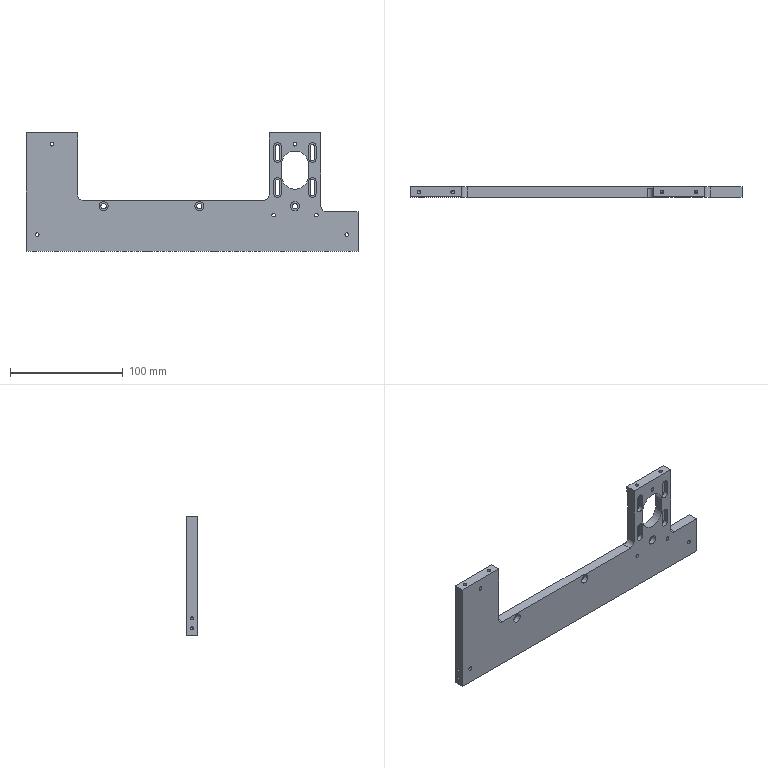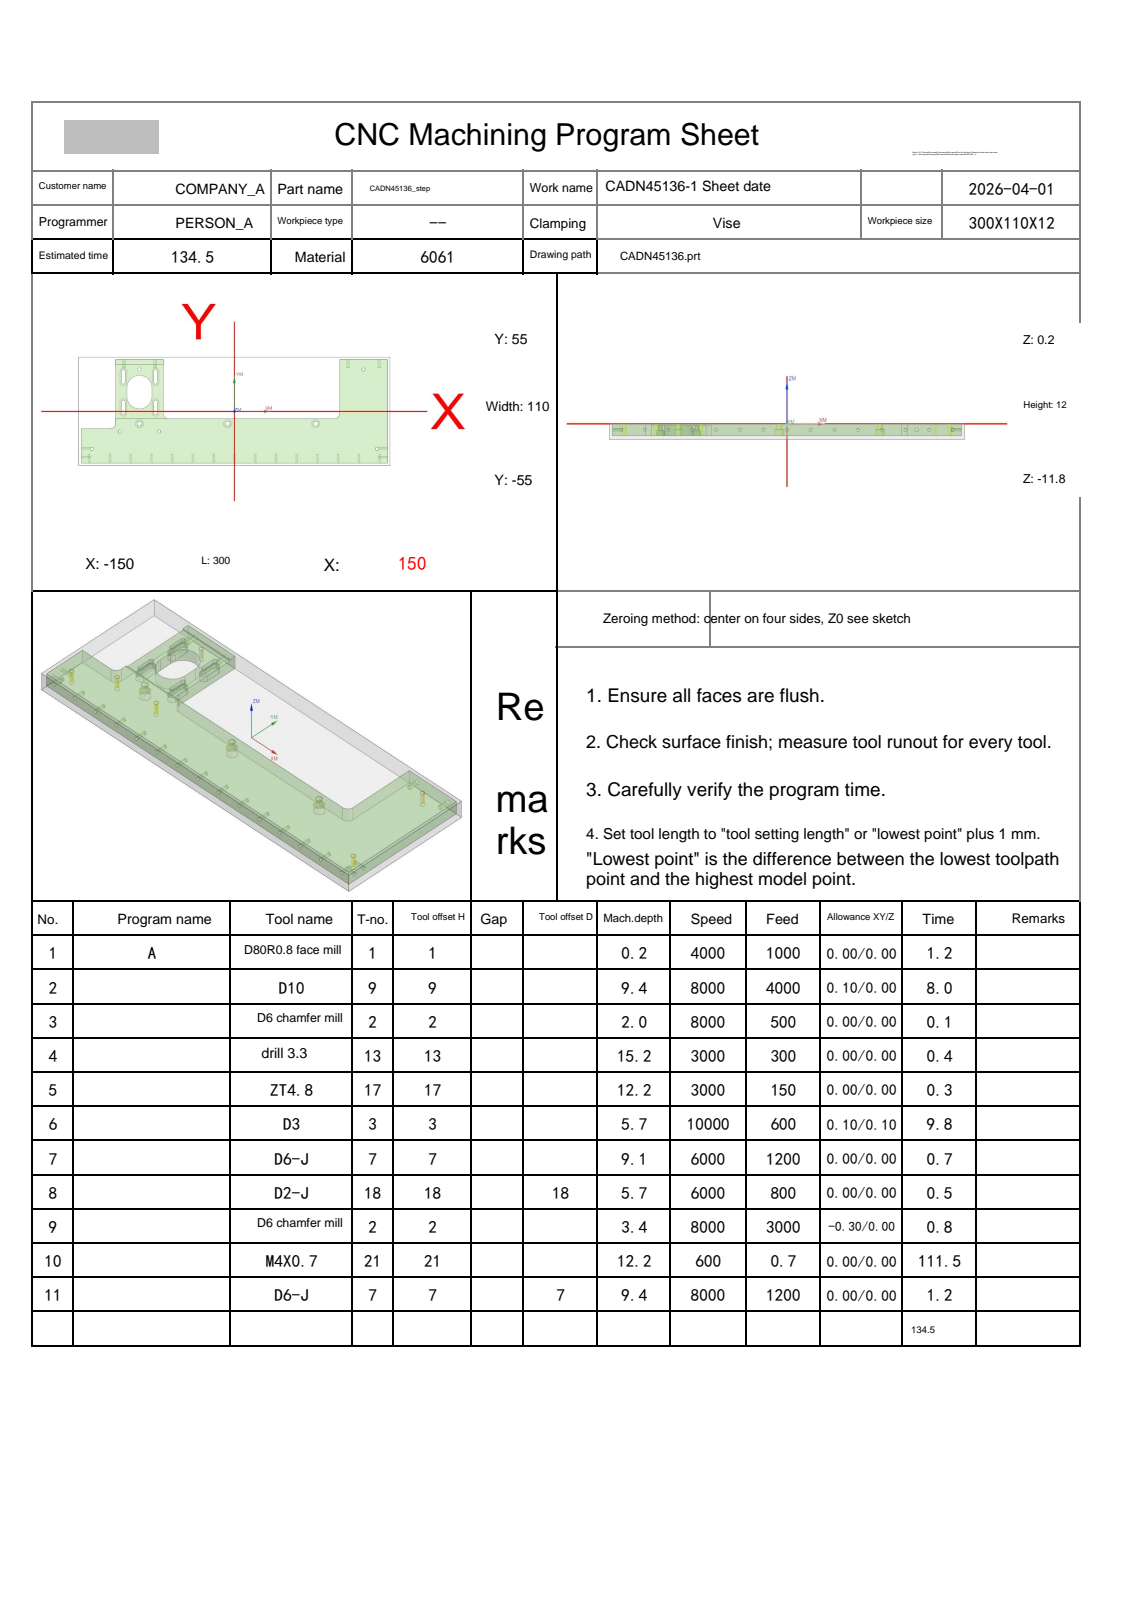NC program | NX | posted by the shop | part box 295 x 9 x 105 mm
Lines 3256 to 4696 of 7463:
N6 T03 M06
(D3  D=3. R=0. H=03 ce=0.10 di=0.10)
G00 G90 G54 X-76.1 Y4. M03 S10000
G43 H03 Z20.
M08
Z-.5
G01 Y-1.55 Z-.519 F600.
X-76.095 Y-1.605
X-76.055 Y-1.645 Z-.52
X-76. Y-1.65
X-75.945 Y-1.645
X-75.905 Y-1.605
X-75.9 Y-1.55
Y9.55 Z-.559
X-75.905 Y9.605
X-75.945 Y9.645
X-76. Y9.65 Z-.56
X-76.055 Y9.645
X-76.095 Y9.605
X-76.1 Y9.55
Y-1.55 Z-.599
X-76.095 Y-1.605
X-76.055 Y-1.645
X-76. Y-1.65
X-75.945 Y-1.645
X-75.905 Y-1.605 Z-.6
X-75.9 Y-1.55
Y9.55 Z-.638
X-75.905 Y9.605 Z-.639
X-75.945 Y9.645
X-76. Y9.65
X-76.055 Y9.645
X-76.095 Y9.605
X-76.1 Y9.55
Y-1.55 Z-.678
X-76.095 Y-1.605
X-76.055 Y-1.645
X-76. Y-1.65 Z-.679
X-75.945 Y-1.645
X-75.905 Y-1.605
X-75.9 Y-1.55
Y9.55 Z-.718
X-75.905 Y9.605
X-75.945 Y9.645
X-76. Y9.65
X-76.055 Y9.645
X-76.095 Y9.605 Z-.719
X-76.1 Y9.55
Y-1.55 Z-.757
X-76.095 Y-1.605 Z-.758
X-76.055 Y-1.645
X-76. Y-1.65
X-75.945 Y-1.645
X-75.905 Y-1.605
X-75.9 Y-1.55
Y9.55 Z-.797
X-75.905 Y9.605
X-75.945 Y9.645
X-76. Y9.65 Z-.798
X-76.055 Y9.645
X-76.095 Y9.605
X-76.1 Y9.55
Y-1.55 Z-.837
X-76.095 Y-1.605
X-76.055 Y-1.645
X-76. Y-1.65
X-75.945 Y-1.645
X-75.905 Y-1.605 Z-.838
X-75.9 Y-1.55
Y9.55 Z-.876
X-75.905 Y9.605 Z-.877
X-75.945 Y9.645
X-76. Y9.65
X-76.055 Y9.645
X-76.095 Y9.605
X-76.1 Y9.55 Z-.878
Y-1.55 Z-.916
X-76.095 Y-1.605
X-76.055 Y-1.645
X-76. Y-1.65 Z-.917
X-75.945 Y-1.645
X-75.905 Y-1.605
X-75.9 Y-1.55
Y9.55 Z-.956
X-75.905 Y9.605
X-75.945 Y9.645
X-76. Y9.65
X-76.055 Y9.645 Z-.957
X-76.095 Y9.605
X-76.1 Y9.55
Y-1.55 Z-.995
X-76.095 Y-1.605 Z-.996
X-76.055 Y-1.645
X-76. Y-1.65
X-75.945 Y-1.645
X-75.905 Y-1.605
X-75.9 Y-1.55 Z-.997
Y9.55 Z-1.035
X-75.905 Y9.605
X-75.945 Y9.645 Z-1.036
X-76. Y9.65
X-76.055 Y9.645
X-76.095 Y9.605
X-76.1 Y9.55
Y-1.55 Z-1.075
X-76.095 Y-1.605
X-76.055 Y-1.645
X-76. Y-1.65
X-75.945 Y-1.645 Z-1.076
X-75.905 Y-1.605
X-75.9 Y-1.55
Y9.55 Z-1.115
X-75.905 Y9.605
X-75.945 Y9.645
X-76. Y9.65
X-76.055 Y9.645
X-76.095 Y9.605
X-76.1 Y9.55 Z-1.116
Y-1.55 Z-1.154
X-76.095 Y-1.605
X-76.055 Y-1.645 Z-1.155
X-76. Y-1.65
X-75.945 Y-1.645
X-75.905 Y-1.605
X-75.9 Y-1.55
Y9.55 Z-1.194
X-75.905 Y9.605
X-75.945 Y9.645
X-76. Y9.65
X-76.055 Y9.645 Z-1.195
X-76.095 Y9.605
X-76.1 Y9.55
Y-1.55 Z-1.234
X-76.095 Y-1.605
X-76.055 Y-1.645
X-76. Y-1.65
X-75.945 Y-1.645
X-75.905 Y-1.605
X-75.9 Y-1.55 Z-1.235
Y9.55 Z-1.273
X-75.905 Y9.605
X-75.945 Y9.645 Z-1.274
X-76. Y9.65
X-76.055 Y9.645
X-76.095 Y9.605
X-76.1 Y9.55
Y-1.55 Z-1.313
X-76.095 Y-1.605
X-76.055 Y-1.645
X-76. Y-1.65
X-75.945 Y-1.645 Z-1.314
X-75.905 Y-1.605
X-75.9 Y-1.55
Y9.55 Z-1.353
X-75.905 Y9.605
X-75.945 Y9.645
X-76. Y9.65
X-76.055 Y9.645
X-76.095 Y9.605 Z-1.354
X-76.1 Y9.55
Y-1.55 Z-1.392
X-76.095 Y-1.605
X-76.055 Y-1.645 Z-1.393
X-76. Y-1.65
X-75.945 Y-1.645
X-75.905 Y-1.605
X-75.9 Y-1.55
Y9.55 Z-1.432
X-75.905 Y9.605
X-75.945 Y9.645
X-76. Y9.65 Z-1.433
X-76.055 Y9.645
X-76.095 Y9.605
X-76.1 Y9.55
Y-1.55 Z-1.472
X-76.095 Y-1.605
X-76.055 Y-1.645
X-76. Y-1.65
X-75.945 Y-1.645
X-75.905 Y-1.605 Z-1.473
X-75.9 Y-1.55
Y9.55 Z-1.511
X-75.905 Y9.605 Z-1.512
X-75.945 Y9.645
X-76. Y9.65
X-76.055 Y9.645
X-76.095 Y9.605
X-76.1 Y9.55
Y-1.55 Z-1.551
X-76.095 Y-1.605
X-76.055 Y-1.645
X-76. Y-1.65 Z-1.552
X-75.945 Y-1.645
X-75.905 Y-1.605
X-75.9 Y-1.55
Y9.55 Z-1.591
X-75.905 Y9.605
X-75.945 Y9.645
X-76. Y9.65
X-76.055 Y9.645
X-76.095 Y9.605 Z-1.592
X-76.1 Y9.55
Y-1.55 Z-1.63
X-76.095 Y-1.605 Z-1.631
X-76.055 Y-1.645
X-76. Y-1.65
X-75.945 Y-1.645
X-75.905 Y-1.605
X-75.9 Y-1.55
Y9.55 Z-1.67
X-75.905 Y9.605
X-75.945 Y9.645
X-76. Y9.65 Z-1.671
X-76.055 Y9.645
X-76.095 Y9.605
X-76.1 Y9.55
Y-1.55 Z-1.71
X-76.095 Y-1.605
X-76.055 Y-1.645
X-76. Y-1.65
X-75.945 Y-1.645 Z-1.711
X-75.905 Y-1.605
X-75.9 Y-1.55
Y9.55 Z-1.749
X-75.905 Y9.605 Z-1.75
X-75.945 Y9.645
X-76. Y9.65
X-76.055 Y9.645
X-76.095 Y9.605
X-76.1 Y9.55 Z-1.751
Y-1.55 Z-1.789
X-76.095 Y-1.605
X-76.055 Y-1.645 Z-1.79
X-76. Y-1.65
X-75.945 Y-1.645
X-75.905 Y-1.605
X-75.9 Y-1.55
Y9.55 Z-1.829
X-75.905 Y9.605
X-75.945 Y9.645
X-76. Y9.65
X-76.055 Y9.645 Z-1.83
X-76.095 Y9.605
X-76.1 Y9.55
Y-1.55 Z-1.869
X-76.095 Y-1.605
X-76.055 Y-1.645
X-76. Y-1.65
X-75.945 Y-1.645
X-75.905 Y-1.605
X-75.9 Y-1.55 Z-1.87
Y9.55 Z-1.908
X-75.905 Y9.605
X-75.945 Y9.645 Z-1.909
X-76. Y9.65
X-76.055 Y9.645
X-76.095 Y9.605
X-76.1 Y9.55
Y-1.55 Z-1.948
X-76.095 Y-1.605
X-76.055 Y-1.645
X-76. Y-1.65
X-75.945 Y-1.645 Z-1.949
X-75.905 Y-1.605
X-75.9 Y-1.55
Y9.55 Z-1.988
X-75.905 Y9.605
X-75.945 Y9.645
X-76. Y9.65
X-76.055 Y9.645
X-76.095 Y9.605
X-76.1 Y9.55 Z-1.989
Y-1.55 Z-2.027
X-76.095 Y-1.605
X-76.055 Y-1.645 Z-2.028
X-76. Y-1.65
X-75.945 Y-1.645
X-75.905 Y-1.605
X-75.9 Y-1.55
Y9.55 Z-2.067
X-75.905 Y9.605
X-75.945 Y9.645
X-76. Y9.65
X-76.055 Y9.645 Z-2.068
X-76.095 Y9.605
X-76.1 Y9.55
Y-1.55 Z-2.107
X-76.095 Y-1.605
X-76.055 Y-1.645
X-76. Y-1.65
X-75.945 Y-1.645
X-75.905 Y-1.605 Z-2.108
X-75.9 Y-1.55
Y9.55 Z-2.146
X-75.905 Y9.605
X-75.945 Y9.645 Z-2.147
X-76. Y9.65
X-76.055 Y9.645
X-76.095 Y9.605
X-76.1 Y9.55
Y-1.55 Z-2.186
X-76.095 Y-1.605
X-76.055 Y-1.645
X-76. Y-1.65 Z-2.187
X-75.945 Y-1.645
X-75.905 Y-1.605
X-75.9 Y-1.55
Y9.55 Z-2.226
X-75.905 Y9.605
X-75.945 Y9.645
X-76. Y9.65
X-76.055 Y9.645
X-76.095 Y9.605 Z-2.227
X-76.1 Y9.55
Y-1.55 Z-2.265
X-76.095 Y-1.605 Z-2.266
X-76.055 Y-1.645
X-76. Y-1.65
X-75.945 Y-1.645
X-75.905 Y-1.605
X-75.9 Y-1.55
Y9.55 Z-2.305
X-75.905 Y9.605
X-75.945 Y9.645
X-76. Y9.65 Z-2.306
X-76.055 Y9.645
X-76.095 Y9.605
X-76.1 Y9.55
Y-1.55 Z-2.345
X-76.095 Y-1.605
X-76.055 Y-1.645
X-76. Y-1.65
X-75.945 Y-1.645
X-75.905 Y-1.605 Z-2.346
X-75.9 Y-1.55
Y9.55 Z-2.384
X-75.905 Y9.605 Z-2.385
X-75.945 Y9.645
X-76. Y9.65
X-76.055 Y9.645
X-76.095 Y9.605
X-76.1 Y9.55
Y-1.55 Z-2.424
X-76.095 Y-1.605
X-76.055 Y-1.645
X-76. Y-1.65 Z-2.425
X-75.945 Y-1.645
X-75.905 Y-1.605
X-75.9 Y-1.55
Y9.55 Z-2.464
X-75.905 Y9.605
X-75.945 Y9.645
X-76. Y9.65
X-76.055 Y9.645
X-76.095 Y9.605 Z-2.465
X-76.1 Y9.55
Y-1.55 Z-2.503
X-76.095 Y-1.605 Z-2.504
X-76.055 Y-1.645
X-76. Y-1.65
X-75.945 Y-1.645
X-75.905 Y-1.605
X-75.9 Y-1.55 Z-2.505
Y9.55 Z-2.543
X-75.905 Y9.605
X-75.945 Y9.645
X-76. Y9.65 Z-2.544
X-76.055 Y9.645
X-76.095 Y9.605
X-76.1 Y9.55
Y-1.55 Z-2.583
X-76.095 Y-1.605
X-76.055 Y-1.645
X-76. Y-1.65
X-75.945 Y-1.645 Z-2.584
X-75.905 Y-1.605
X-75.9 Y-1.55
Y9.55 Z-2.622
X-75.905 Y9.605 Z-2.623
X-75.945 Y9.645
X-76. Y9.65
X-76.055 Y9.645
X-76.095 Y9.605
X-76.1 Y9.55 Z-2.624
Y-1.55 Z-2.662
X-76.095 Y-1.605
X-76.055 Y-1.645 Z-2.663
X-76. Y-1.65
X-75.945 Y-1.645
X-75.905 Y-1.605
X-75.9 Y-1.55
Y9.55 Z-2.702
X-75.905 Y9.605
X-75.945 Y9.645
X-76. Y9.65
X-76.055 Y9.645 Z-2.703
X-76.095 Y9.605
X-76.1 Y9.55
Y-1.55 Z-2.742
X-76.095 Y-1.605
X-76.055 Y-1.645
X-76. Y-1.65
X-75.945 Y-1.645
X-75.905 Y-1.605
X-75.9 Y-1.55 Z-2.743
Y9.55 Z-2.781
X-75.905 Y9.605
X-75.945 Y9.645 Z-2.782
X-76. Y9.65
X-76.055 Y9.645
X-76.095 Y9.605
X-76.1 Y9.55
Y-1.55 Z-2.821
X-76.095 Y-1.605
X-76.055 Y-1.645
X-76. Y-1.65
X-75.945 Y-1.645 Z-2.822
X-75.905 Y-1.605
X-75.9 Y-1.55
Y9.55 Z-2.861
X-75.905 Y9.605
X-75.945 Y9.645
X-76. Y9.65
X-76.055 Y9.645
X-76.095 Y9.605
X-76.1 Y9.55 Z-2.862
Y-1.55 Z-2.9
X-76.095 Y-1.605
X-76.055 Y-1.645 Z-2.901
X-76. Y-1.65
X-75.945 Y-1.645
X-75.905 Y-1.605
X-75.9 Y-1.55
Y9.55 Z-2.94
X-75.905 Y9.605
X-75.945 Y9.645
X-76. Y9.65
X-76.055 Y9.645 Z-2.941
X-76.095 Y9.605
X-76.1 Y9.55
Y-1.55 Z-2.98
X-76.095 Y-1.605
X-76.055 Y-1.645
X-76. Y-1.65
X-75.945 Y-1.645
X-75.905 Y-1.605 Z-2.981
X-75.9 Y-1.55
Y9.55 Z-3.019
X-75.905 Y9.605
X-75.945 Y9.645 Z-3.02
X-76. Y9.65
X-76.055 Y9.645
X-76.095 Y9.605
X-76.1 Y9.55
Y-1.55 Z-3.059
X-76.095 Y-1.605
X-76.055 Y-1.645
X-76. Y-1.65 Z-3.06
X-75.945 Y-1.645
X-75.905 Y-1.605
X-75.9 Y-1.55
Y9.55 Z-3.099
X-75.905 Y9.605
X-75.945 Y9.645
X-76. Y9.65
X-76.055 Y9.645
X-76.095 Y9.605 Z-3.1
X-76.1 Y9.55
Y-1.55 Z-3.138
X-76.095 Y-1.605 Z-3.139
X-76.055 Y-1.645
X-76. Y-1.65
X-75.945 Y-1.645
X-75.905 Y-1.605
X-75.9 Y-1.55
Y9.55 Z-3.178
X-75.905 Y9.605
X-75.945 Y9.645
X-76. Y9.65 Z-3.179
X-76.055 Y9.645
X-76.095 Y9.605
X-76.1 Y9.55
Y-1.55 Z-3.218
X-76.095 Y-1.605
X-76.055 Y-1.645
X-76. Y-1.65
X-75.945 Y-1.645
X-75.905 Y-1.605 Z-3.219
X-75.9 Y-1.55
Y9.55 Z-3.257
X-75.905 Y9.605 Z-3.258
X-75.945 Y9.645
X-76. Y9.65
X-76.055 Y9.645
X-76.095 Y9.605
X-76.1 Y9.55
Y-1.55 Z-3.297
X-76.095 Y-1.605
X-76.055 Y-1.645
X-76. Y-1.65 Z-3.298
X-75.945 Y-1.645
X-75.905 Y-1.605
X-75.9 Y-1.55
Y9.55 Z-3.337
X-75.905 Y9.605
X-75.945 Y9.645
X-76. Y9.65
X-76.055 Y9.645
X-76.095 Y9.605 Z-3.338
X-76.1 Y9.55
Y-1.55 Z-3.376
X-76.095 Y-1.605 Z-3.377
X-76.055 Y-1.645
X-76. Y-1.65
X-75.945 Y-1.645
X-75.905 Y-1.605
X-75.9 Y-1.55 Z-3.378
Y9.55 Z-3.416
X-75.905 Y9.605
X-75.945 Y9.645
X-76. Y9.65 Z-3.417
X-76.055 Y9.645
X-76.095 Y9.605
X-76.1 Y9.55
Y-1.55 Z-3.456
X-76.095 Y-1.605
X-76.055 Y-1.645
X-76. Y-1.65
X-75.945 Y-1.645 Z-3.457
X-75.905 Y-1.605
X-75.9 Y-1.55
Y9.55 Z-3.495
X-75.905 Y9.605 Z-3.496
X-75.945 Y9.645
X-76. Y9.65
X-76.055 Y9.645
X-76.095 Y9.605
X-76.1 Y9.55 Z-3.497
Y-1.55 Z-3.535
X-76.095 Y-1.605
X-76.055 Y-1.645 Z-3.536
X-76. Y-1.65
X-75.945 Y-1.645
X-75.905 Y-1.605
X-75.9 Y-1.55
Y9.55 Z-3.575
X-75.905 Y9.605
X-75.945 Y9.645
X-76. Y9.65
X-76.055 Y9.645 Z-3.576
X-76.095 Y9.605
X-76.1 Y9.55
Y-1.55 Z-3.615
X-76.095 Y-1.605
X-76.055 Y-1.645
X-76. Y-1.65
X-75.945 Y-1.645
X-75.905 Y-1.605
X-75.9 Y-1.55 Z-3.616
Y9.55 Z-3.654
X-75.905 Y9.605
X-75.945 Y9.645 Z-3.655
X-76. Y9.65
X-76.055 Y9.645
X-76.095 Y9.605
X-76.1 Y9.55
Y-1.55 Z-3.694
X-76.095 Y-1.605
X-76.055 Y-1.645
X-76. Y-1.65
X-75.945 Y-1.645 Z-3.695
X-75.905 Y-1.605
X-75.9 Y-1.55
Y9.55 Z-3.734
X-75.905 Y9.605
X-75.945 Y9.645
X-76. Y9.65
X-76.055 Y9.645
X-76.095 Y9.605
X-76.1 Y9.55 Z-3.735
Y-1.55 Z-3.773
X-76.095 Y-1.605
X-76.055 Y-1.645 Z-3.774
X-76. Y-1.65
X-75.945 Y-1.645
X-75.905 Y-1.605
X-75.9 Y-1.55
Y9.55 Z-3.813
X-75.905 Y9.605
X-75.945 Y9.645
X-76. Y9.65
X-76.055 Y9.645 Z-3.814
X-76.095 Y9.605
X-76.1 Y9.55
Y-1.55 Z-3.853
X-76.095 Y-1.605
X-76.055 Y-1.645
X-76. Y-1.65
X-75.945 Y-1.645
X-75.905 Y-1.605 Z-3.854
X-75.9 Y-1.55
Y9.55 Z-3.892
X-75.905 Y9.605
X-75.945 Y9.645 Z-3.893
X-76. Y9.65
X-76.055 Y9.645
X-76.095 Y9.605
X-76.1 Y9.55
Y-1.55 Z-3.932
X-76.095 Y-1.605
X-76.055 Y-1.645
X-76. Y-1.65 Z-3.933
X-75.945 Y-1.645
X-75.905 Y-1.605
X-75.9 Y-1.55
Y9.55 Z-3.972
X-75.905 Y9.605
X-75.945 Y9.645
X-76. Y9.65
X-76.055 Y9.645
X-76.095 Y9.605 Z-3.973
X-76.1 Y9.55
Y-1.55 Z-4.011
X-76.095 Y-1.605 Z-4.012
X-76.055 Y-1.645
X-76. Y-1.65
X-75.945 Y-1.645
X-75.905 Y-1.605
X-75.9 Y-1.55
Y9.55 Z-4.051
X-75.905 Y9.605
X-75.945 Y9.645
X-76. Y9.65 Z-4.052
X-76.055 Y9.645
X-76.095 Y9.605
X-76.1 Y9.55
Y-1.55 Z-4.091
X-76.095 Y-1.605
X-76.055 Y-1.645
X-76. Y-1.65
X-75.945 Y-1.645
X-75.905 Y-1.605 Z-4.092
X-75.9 Y-1.55
Y9.55 Z-4.13
X-75.905 Y9.605 Z-4.131
X-75.945 Y9.645
X-76. Y9.65
X-76.055 Y9.645
X-76.095 Y9.605
X-76.1 Y9.55
Y-1.55 Z-4.17
X-76.095 Y-1.605
X-76.055 Y-1.645
X-76. Y-1.65 Z-4.171
X-75.945 Y-1.645
X-75.905 Y-1.605
X-75.9 Y-1.55
Y9.55 Z-4.21
X-75.905 Y9.605
X-75.945 Y9.645
X-76. Y9.65
X-76.055 Y9.645 Z-4.211
X-76.095 Y9.605
X-76.1 Y9.55
Y-1.55 Z-4.249
X-76.095 Y-1.605 Z-4.25
X-76.055 Y-1.645
X-76. Y-1.65
X-75.945 Y-1.645
X-75.905 Y-1.605
X-75.9 Y-1.55 Z-4.251
Y9.55 Z-4.289
X-75.905 Y9.605
X-75.945 Y9.645 Z-4.29
X-76. Y9.65
X-76.055 Y9.645
X-76.095 Y9.605
X-76.1 Y9.55
Y-1.55 Z-4.329
X-76.095 Y-1.605
X-76.055 Y-1.645
X-76. Y-1.65
X-75.945 Y-1.645 Z-4.33
X-75.905 Y-1.605
X-75.9 Y-1.55
Y9.55 Z-4.369
X-75.905 Y9.605
X-75.945 Y9.645
X-76. Y9.65
X-76.055 Y9.645
X-76.095 Y9.605
X-76.1 Y9.55 Z-4.37
Y-1.55 Z-4.408
X-76.095 Y-1.605
X-76.055 Y-1.645 Z-4.409
X-76. Y-1.65
X-75.945 Y-1.645
X-75.905 Y-1.605
X-75.9 Y-1.55
Y9.55 Z-4.448
X-75.905 Y9.605
X-75.945 Y9.645
X-76. Y9.65
X-76.055 Y9.645 Z-4.449
X-76.095 Y9.605
X-76.1 Y9.55
Y-1.55 Z-4.488
X-76.095 Y-1.605
X-76.055 Y-1.645
X-76. Y-1.65
X-75.945 Y-1.645
X-75.905 Y-1.605
X-75.9 Y-1.55 Z-4.489
Y9.55 Z-4.527
X-75.905 Y9.605
X-75.945 Y9.645 Z-4.528
X-76. Y9.65
X-76.055 Y9.645
X-76.095 Y9.605
X-76.1 Y9.55
Y-1.55 Z-4.567
X-76.095 Y-1.605
X-76.055 Y-1.645
X-76. Y-1.65
X-75.945 Y-1.645 Z-4.568
X-75.905 Y-1.605
X-75.9 Y-1.55
Y9.55 Z-4.607
X-75.905 Y9.605
X-75.945 Y9.645
X-76. Y9.65
X-76.055 Y9.645
X-76.095 Y9.605 Z-4.608
X-76.1 Y9.55
Y-1.55 Z-4.646
X-76.095 Y-1.605
X-76.055 Y-1.645 Z-4.647
X-76. Y-1.65
X-75.945 Y-1.645
X-75.905 Y-1.605
X-75.9 Y-1.55
Y9.55 Z-4.686
X-75.905 Y9.605
X-75.945 Y9.645
X-76. Y9.65 Z-4.687
X-76.055 Y9.645
X-76.095 Y9.605
X-76.1 Y9.55
Y-1.55 Z-4.726
X-76.095 Y-1.605
X-76.055 Y-1.645
X-76. Y-1.65
X-75.945 Y-1.645
X-75.905 Y-1.605 Z-4.727
X-75.9 Y-1.55
Y9.55 Z-4.765
X-75.905 Y9.605 Z-4.766
X-75.945 Y9.645
X-76. Y9.65
X-76.055 Y9.645
X-76.095 Y9.605
X-76.1 Y9.55
Y-1.55 Z-4.805
X-76.095 Y-1.605
X-76.055 Y-1.645
X-76. Y-1.65 Z-4.806
X-75.945 Y-1.645
X-75.905 Y-1.605
X-75.9 Y-1.55
Y9.55 Z-4.845
X-75.905 Y9.605
X-75.945 Y9.645
X-76. Y9.65
X-76.055 Y9.645
X-76.095 Y9.605 Z-4.846
X-76.1 Y9.55
Y-1.55 Z-4.884
X-76.095 Y-1.605 Z-4.885
X-76.055 Y-1.645
X-76. Y-1.65
X-75.945 Y-1.645
X-75.905 Y-1.605
X-75.9 Y-1.55
Y9.55 Z-4.924
X-75.905 Y9.605
X-75.945 Y9.645
X-76. Y9.65 Z-4.925
X-76.055 Y9.645
X-76.095 Y9.605
X-76.1 Y9.55
Y-1.55 Z-4.964
X-76.095 Y-1.605
X-76.055 Y-1.645
X-76. Y-1.65
X-75.945 Y-1.645
X-75.905 Y-1.605 Z-4.965
X-75.9 Y-1.55
Y9.55 Z-5.003
X-75.905 Y9.605 Z-5.004
X-75.945 Y9.645
X-76. Y9.65
X-76.055 Y9.645
X-76.095 Y9.605
X-76.1 Y9.55 Z-5.005
Y-1.55 Z-5.043
X-76.095 Y-1.605
X-76.055 Y-1.645
X-76. Y-1.65 Z-5.044
X-75.945 Y-1.645
X-75.905 Y-1.605
X-75.9 Y-1.55
Y9.55 Z-5.083
X-75.905 Y9.605
X-75.945 Y9.645
X-76. Y9.65
X-76.055 Y9.645 Z-5.084
X-76.095 Y9.605
X-76.1 Y9.55
Y-1.55 Z-5.122
X-76.095 Y-1.605 Z-5.123
X-76.055 Y-1.645
X-76. Y-1.65
X-75.945 Y-1.645
X-75.905 Y-1.605
X-75.9 Y-1.55 Z-5.124
Y9.55 Z-5.162
X-75.905 Y9.605
X-75.945 Y9.645 Z-5.163
X-76. Y9.65
X-76.055 Y9.645
X-76.095 Y9.605
X-76.1 Y9.55
Y-1.55 Z-5.202
X-76.095 Y-1.605
X-76.055 Y-1.645
X-76. Y-1.65
X-75.945 Y-1.645 Z-5.203
X-75.905 Y-1.605
X-75.9 Y-1.55
Y9.55 Z-5.242
X-75.905 Y9.605
X-75.945 Y9.645
X-76. Y9.65
X-76.055 Y9.645
X-76.095 Y9.605
X-76.1 Y9.55 Z-5.243
Y-1.55 Z-5.281
X-76.095 Y-1.605
X-76.055 Y-1.645 Z-5.282
X-76. Y-1.65
X-75.945 Y-1.645
X-75.905 Y-1.605
X-75.9 Y-1.55
Y9.55 Z-5.321
X-75.905 Y9.605
X-75.945 Y9.645
X-76. Y9.65
X-76.055 Y9.645 Z-5.322
X-76.095 Y9.605
X-76.1 Y9.55
Y-1.55 Z-5.361
X-76.095 Y-1.605
X-76.055 Y-1.645
X-76. Y-1.65
X-75.945 Y-1.645
X-75.905 Y-1.605
X-75.9 Y-1.55 Z-5.362
Y9.55 Z-5.4
X-75.905 Y9.605
X-75.945 Y9.645 Z-5.401
X-76. Y9.65
X-76.055 Y9.645
X-76.095 Y9.605
X-76.1 Y9.55
Y-1.55 Z-5.44
X-76.095 Y-1.605
X-76.055 Y-1.645
X-76. Y-1.65
X-75.945 Y-1.645 Z-5.441
X-75.905 Y-1.605
X-75.9 Y-1.55
Y9.55 Z-5.48
X-75.905 Y9.605
X-75.945 Y9.645
X-76. Y9.65
X-76.055 Y9.645
X-76.095 Y9.605 Z-5.481
X-76.1 Y9.55
Y4. Z-5.5
Y-1.55
X-76. Y-1.65
X-75.9 Y-1.55
Y9.55
X-76. Y9.65
X-76.1 Y9.55
Y4.
Y3.5
Z-4.5
G00 Z20.
X-107.1 Y4.
Z-.5
G01 Y-1.55 Z-.519
X-107.095 Y-1.605
X-107.055 Y-1.645 Z-.52
X-107. Y-1.65
X-106.945 Y-1.645
X-106.905 Y-1.605
X-106.9 Y-1.55
Y9.55 Z-.559
X-106.905 Y9.605
X-106.945 Y9.645
X-107. Y9.65 Z-.56
X-107.055 Y9.645
X-107.095 Y9.605
X-107.1 Y9.55
Y-1.55 Z-.599
X-107.095 Y-1.605
X-107.055 Y-1.645
X-107. Y-1.65
X-106.945 Y-1.645
X-106.905 Y-1.605 Z-.6
X-106.9 Y-1.55
Y9.55 Z-.638
X-106.905 Y9.605 Z-.639
X-106.945 Y9.645
X-107. Y9.65
X-107.055 Y9.645
X-107.095 Y9.605
X-107.1 Y9.55
Y-1.55 Z-.678
X-107.095 Y-1.605
X-107.055 Y-1.645
X-107. Y-1.65 Z-.679
X-106.945 Y-1.645
X-106.905 Y-1.605
X-106.9 Y-1.55
Y9.55 Z-.718
X-106.905 Y9.605
X-106.945 Y9.645
X-107. Y9.65
X-107.055 Y9.645
X-107.095 Y9.605 Z-.719
X-107.1 Y9.55
Y-1.55 Z-.757
X-107.095 Y-1.605 Z-.758
X-107.055 Y-1.645
X-107. Y-1.65
X-106.945 Y-1.645
X-106.905 Y-1.605
X-106.9 Y-1.55
Y9.55 Z-.797
X-106.905 Y9.605
X-106.945 Y9.645
X-107. Y9.65 Z-.798
X-107.055 Y9.645
X-107.095 Y9.605
X-107.1 Y9.55
Y-1.55 Z-.837
X-107.095 Y-1.605
X-107.055 Y-1.645
X-107. Y-1.65
X-106.945 Y-1.645
X-106.905 Y-1.605 Z-.838
X-106.9 Y-1.55
Y9.55 Z-.876
X-106.905 Y9.605 Z-.877
X-106.945 Y9.645
X-107. Y9.65
X-107.055 Y9.645
X-107.095 Y9.605
X-107.1 Y9.55 Z-.878
Y-1.55 Z-.916
X-107.095 Y-1.605
X-107.055 Y-1.645
X-107. Y-1.65 Z-.917
X-106.945 Y-1.645
X-106.905 Y-1.605
X-106.9 Y-1.55
Y9.55 Z-.956
X-106.905 Y9.605
X-106.945 Y9.645
X-107. Y9.65
X-107.055 Y9.645 Z-.957
X-107.095 Y9.605
X-107.1 Y9.55
Y-1.55 Z-.995
X-107.095 Y-1.605 Z-.996
X-107.055 Y-1.645
X-107. Y-1.65
X-106.945 Y-1.645
X-106.905 Y-1.605
X-106.9 Y-1.55 Z-.997
Y9.55 Z-1.035
X-106.905 Y9.605
X-106.945 Y9.645 Z-1.036
X-107. Y9.65
X-107.055 Y9.645
X-107.095 Y9.605
X-107.1 Y9.55
Y-1.55 Z-1.075
X-107.095 Y-1.605
X-107.055 Y-1.645
X-107. Y-1.65
X-106.945 Y-1.645 Z-1.076
X-106.905 Y-1.605
X-106.9 Y-1.55
Y9.55 Z-1.115
X-106.905 Y9.605
X-106.945 Y9.645
X-107. Y9.65
X-107.055 Y9.645
X-107.095 Y9.605
X-107.1 Y9.55 Z-1.116
Y-1.55 Z-1.154
X-107.095 Y-1.605
X-107.055 Y-1.645 Z-1.155
X-107. Y-1.65
X-106.945 Y-1.645
X-106.905 Y-1.605
X-106.9 Y-1.55
Y9.55 Z-1.194
X-106.905 Y9.605
X-106.945 Y9.645
X-107. Y9.65
X-107.055 Y9.645 Z-1.195
X-107.095 Y9.605
X-107.1 Y9.55
Y-1.55 Z-1.234
X-107.095 Y-1.605
X-107.055 Y-1.645
X-107. Y-1.65
X-106.945 Y-1.645
X-106.905 Y-1.605
X-106.9 Y-1.55 Z-1.235
Y9.55 Z-1.273
X-106.905 Y9.605
X-106.945 Y9.645 Z-1.274
X-107. Y9.65
X-107.055 Y9.645
X-107.095 Y9.605
X-107.1 Y9.55
Y-1.55 Z-1.313
X-107.095 Y-1.605
X-107.055 Y-1.645
X-107. Y-1.65
X-106.945 Y-1.645 Z-1.314
X-106.905 Y-1.605
X-106.9 Y-1.55
Y9.55 Z-1.353
X-106.905 Y9.605
X-106.945 Y9.645
X-107. Y9.65
X-107.055 Y9.645
X-107.095 Y9.605 Z-1.354
X-107.1 Y9.55
Y-1.55 Z-1.392
X-107.095 Y-1.605
X-107.055 Y-1.645 Z-1.393
X-107. Y-1.65
X-106.945 Y-1.645
X-106.905 Y-1.605
X-106.9 Y-1.55
Y9.55 Z-1.432
X-106.905 Y9.605
X-106.945 Y9.645
X-107. Y9.65 Z-1.433
X-107.055 Y9.645
X-107.095 Y9.605
X-107.1 Y9.55
Y-1.55 Z-1.472
X-107.095 Y-1.605
X-107.055 Y-1.645
X-107. Y-1.65
X-106.945 Y-1.645
X-106.905 Y-1.605 Z-1.473
X-106.9 Y-1.55
Y9.55 Z-1.511
X-106.905 Y9.605 Z-1.512
X-106.945 Y9.645
X-107. Y9.65
X-107.055 Y9.645
X-107.095 Y9.605
X-107.1 Y9.55
Y-1.55 Z-1.551
X-107.095 Y-1.605
X-107.055 Y-1.645
X-107. Y-1.65 Z-1.552
X-106.945 Y-1.645
X-106.905 Y-1.605
X-106.9 Y-1.55
Y9.55 Z-1.591
X-106.905 Y9.605
X-106.945 Y9.645
X-107. Y9.65
X-107.055 Y9.645
X-107.095 Y9.605 Z-1.592
X-107.1 Y9.55
Y-1.55 Z-1.63
X-107.095 Y-1.605 Z-1.631
X-107.055 Y-1.645
X-107. Y-1.65
X-106.945 Y-1.645
X-106.905 Y-1.605
X-106.9 Y-1.55
Y9.55 Z-1.67
X-106.905 Y9.605
X-106.945 Y9.645
X-107. Y9.65 Z-1.671
X-107.055 Y9.645
X-107.095 Y9.605
X-107.1 Y9.55
Y-1.55 Z-1.71
X-107.095 Y-1.605
X-107.055 Y-1.645
X-107. Y-1.65
X-106.945 Y-1.645 Z-1.711
X-106.905 Y-1.605
X-106.9 Y-1.55
Y9.55 Z-1.749
X-106.905 Y9.605 Z-1.75
X-106.945 Y9.645
X-107. Y9.65
X-107.055 Y9.645
X-107.095 Y9.605
X-107.1 Y9.55 Z-1.751
Y-1.55 Z-1.789
X-107.095 Y-1.605
X-107.055 Y-1.645 Z-1.79
X-107. Y-1.65
X-106.945 Y-1.645
X-106.905 Y-1.605
X-106.9 Y-1.55
Y9.55 Z-1.829
X-106.905 Y9.605
X-106.945 Y9.645
X-107. Y9.65
X-107.055 Y9.645 Z-1.83
X-107.095 Y9.605
X-107.1 Y9.55
Y-1.55 Z-1.869
X-107.095 Y-1.605
X-107.055 Y-1.645
X-107. Y-1.65
X-106.945 Y-1.645
X-106.905 Y-1.605
X-106.9 Y-1.55 Z-1.87
Y9.55 Z-1.908
X-106.905 Y9.605
X-106.945 Y9.645 Z-1.909
X-107. Y9.65
X-107.055 Y9.645
X-107.095 Y9.605
X-107.1 Y9.55
Y-1.55 Z-1.948
X-107.095 Y-1.605
X-107.055 Y-1.645
X-107. Y-1.65
X-106.945 Y-1.645 Z-1.949
X-106.905 Y-1.605
X-106.9 Y-1.55
Y9.55 Z-1.988
X-106.905 Y9.605
X-106.945 Y9.645
X-107. Y9.65
X-107.055 Y9.645
X-107.095 Y9.605
X-107.1 Y9.55 Z-1.989
Y-1.55 Z-2.027
X-107.095 Y-1.605
X-107.055 Y-1.645 Z-2.028
X-107. Y-1.65
X-106.945 Y-1.645
X-106.905 Y-1.605
X-106.9 Y-1.55
Y9.55 Z-2.067
X-106.905 Y9.605
X-106.945 Y9.645
X-107. Y9.65
X-107.055 Y9.645 Z-2.068
X-107.095 Y9.605
X-107.1 Y9.55
Y-1.55 Z-2.107
X-107.095 Y-1.605
X-107.055 Y-1.645
X-107. Y-1.65
X-106.945 Y-1.645
X-106.905 Y-1.605 Z-2.108
X-106.9 Y-1.55
Y9.55 Z-2.146
X-106.905 Y9.605
X-106.945 Y9.645 Z-2.147
X-107. Y9.65
X-107.055 Y9.645
X-107.095 Y9.605
X-107.1 Y9.55
Y-1.55 Z-2.186
X-107.095 Y-1.605
X-107.055 Y-1.645
X-107. Y-1.65 Z-2.187
X-106.945 Y-1.645
X-106.905 Y-1.605
X-106.9 Y-1.55
Y9.55 Z-2.226
X-106.905 Y9.605
X-106.945 Y9.645
X-107. Y9.65
X-107.055 Y9.645
X-107.095 Y9.605 Z-2.227
X-107.1 Y9.55
Y-1.55 Z-2.265
X-107.095 Y-1.605 Z-2.266
X-107.055 Y-1.645
X-107. Y-1.65
X-106.945 Y-1.645
X-106.905 Y-1.605
X-106.9 Y-1.55
Y9.55 Z-2.305
X-106.905 Y9.605
X-106.945 Y9.645
X-107. Y9.65 Z-2.306
X-107.055 Y9.645
X-107.095 Y9.605
X-107.1 Y9.55
Y-1.55 Z-2.345
X-107.095 Y-1.605
X-107.055 Y-1.645
X-107. Y-1.65
X-106.945 Y-1.645
X-106.905 Y-1.605 Z-2.346
X-106.9 Y-1.55
Y9.55 Z-2.384
X-106.905 Y9.605 Z-2.385
X-106.945 Y9.645
X-107. Y9.65
X-107.055 Y9.645
X-107.095 Y9.605
X-107.1 Y9.55
Y-1.55 Z-2.424
X-107.095 Y-1.605
X-107.055 Y-1.645
X-107. Y-1.65 Z-2.425
X-106.945 Y-1.645
X-106.905 Y-1.605
X-106.9 Y-1.55
Y9.55 Z-2.464
X-106.905 Y9.605
X-106.945 Y9.645
X-107. Y9.65
X-107.055 Y9.645
X-107.095 Y9.605 Z-2.465
X-107.1 Y9.55
Y-1.55 Z-2.503
X-107.095 Y-1.605 Z-2.504
X-107.055 Y-1.645
X-107. Y-1.65
X-106.945 Y-1.645
X-106.905 Y-1.605
X-106.9 Y-1.55 Z-2.505
Y9.55 Z-2.543
X-106.905 Y9.605
X-106.945 Y9.645
X-107. Y9.65 Z-2.544
X-107.055 Y9.645
X-107.095 Y9.605
X-107.1 Y9.55
Y-1.55 Z-2.583
X-107.095 Y-1.605
X-107.055 Y-1.645
X-107. Y-1.65
X-106.945 Y-1.645 Z-2.584
X-106.905 Y-1.605
X-106.9 Y-1.55
Y9.55 Z-2.622
X-106.905 Y9.605 Z-2.623
X-106.945 Y9.645
X-107. Y9.65
X-107.055 Y9.645
X-107.095 Y9.605
X-107.1 Y9.55 Z-2.624
Y-1.55 Z-2.662
X-107.095 Y-1.605
X-107.055 Y-1.645 Z-2.663
X-107. Y-1.65
X-106.945 Y-1.645
X-106.905 Y-1.605
X-106.9 Y-1.55
Y9.55 Z-2.702
X-106.905 Y9.605
X-106.945 Y9.645
X-107. Y9.65
X-107.055 Y9.645 Z-2.703
X-107.095 Y9.605
X-107.1 Y9.55
Y-1.55 Z-2.742
X-107.095 Y-1.605
X-107.055 Y-1.645
X-107. Y-1.65
X-106.945 Y-1.645
X-106.905 Y-1.605
X-106.9 Y-1.55 Z-2.743
Y9.55 Z-2.781
X-106.905 Y9.605
X-106.945 Y9.645 Z-2.782
X-107. Y9.65
X-107.055 Y9.645
X-107.095 Y9.605
X-107.1 Y9.55
Y-1.55 Z-2.821
X-107.095 Y-1.605
X-107.055 Y-1.645
X-107. Y-1.65
X-106.945 Y-1.645 Z-2.822
X-106.905 Y-1.605
X-106.9 Y-1.55
Y9.55 Z-2.861
X-106.905 Y9.605
X-106.945 Y9.645
X-107. Y9.65
X-107.055 Y9.645
X-107.095 Y9.605
X-107.1 Y9.55 Z-2.862
Y-1.55 Z-2.9
X-107.095 Y-1.605
X-107.055 Y-1.645 Z-2.901
X-107. Y-1.65
X-106.945 Y-1.645
X-106.905 Y-1.605
X-106.9 Y-1.55
Y9.55 Z-2.94
X-106.905 Y9.605
X-106.945 Y9.645
X-107. Y9.65
X-107.055 Y9.645 Z-2.941
X-107.095 Y9.605
X-107.1 Y9.55
Y-1.55 Z-2.98
X-107.095 Y-1.605
X-107.055 Y-1.645
X-107. Y-1.65
X-106.945 Y-1.645
X-106.905 Y-1.605 Z-2.981
X-106.9 Y-1.55
Y9.55 Z-3.019
X-106.905 Y9.605
X-106.945 Y9.645 Z-3.02
X-107. Y9.65
X-107.055 Y9.645
X-107.095 Y9.605
X-107.1 Y9.55
Y-1.55 Z-3.059
X-107.095 Y-1.605
X-107.055 Y-1.645
X-107. Y-1.65 Z-3.06
X-106.945 Y-1.645
X-106.905 Y-1.605
X-106.9 Y-1.55
Y9.55 Z-3.099
X-106.905 Y9.605
X-106.945 Y9.645
X-107. Y9.65
X-107.055 Y9.645
X-107.095 Y9.605 Z-3.1
X-107.1 Y9.55
Y-1.55 Z-3.138
X-107.095 Y-1.605 Z-3.139
X-107.055 Y-1.645
X-107. Y-1.65
X-106.945 Y-1.645
X-106.905 Y-1.605
X-106.9 Y-1.55
Y9.55 Z-3.178
X-106.905 Y9.605
X-106.945 Y9.645
X-107. Y9.65 Z-3.179
X-107.055 Y9.645
X-107.095 Y9.605
X-107.1 Y9.55
Y-1.55 Z-3.218
X-107.095 Y-1.605
X-107.055 Y-1.645
X-107. Y-1.65
X-106.945 Y-1.645
X-106.905 Y-1.605 Z-3.219
X-106.9 Y-1.55
Y9.55 Z-3.257
X-106.905 Y9.605 Z-3.258
X-106.945 Y9.645
X-107. Y9.65
X-107.055 Y9.645
X-107.095 Y9.605
X-107.1 Y9.55
Y-1.55 Z-3.297
X-107.095 Y-1.605
X-107.055 Y-1.645
X-107. Y-1.65 Z-3.298
X-106.945 Y-1.645
X-106.905 Y-1.605
X-106.9 Y-1.55
Y9.55 Z-3.337
X-106.905 Y9.605
X-106.945 Y9.645
X-107. Y9.65
X-107.055 Y9.645
X-107.095 Y9.605 Z-3.338
X-107.1 Y9.55
Y-1.55 Z-3.376
X-107.095 Y-1.605 Z-3.377
X-107.055 Y-1.645
X-107. Y-1.65
X-106.945 Y-1.645
X-106.905 Y-1.605
X-106.9 Y-1.55 Z-3.378
Y9.55 Z-3.416
X-106.905 Y9.605
X-106.945 Y9.645
X-107. Y9.65 Z-3.417
X-107.055 Y9.645
X-107.095 Y9.605
X-107.1 Y9.55
Y-1.55 Z-3.456
X-107.095 Y-1.605
X-107.055 Y-1.645
X-107. Y-1.65
X-106.945 Y-1.645 Z-3.457
X-106.905 Y-1.605
X-106.9 Y-1.55
Y9.55 Z-3.495
X-106.905 Y9.605 Z-3.496
X-106.945 Y9.645
X-107. Y9.65
X-107.055 Y9.645
X-107.095 Y9.605
X-107.1 Y9.55 Z-3.497
Y-1.55 Z-3.535
X-107.095 Y-1.605
X-107.055 Y-1.645 Z-3.536
X-107. Y-1.65
X-106.945 Y-1.645
X-106.905 Y-1.605
X-106.9 Y-1.55
Y9.55 Z-3.575